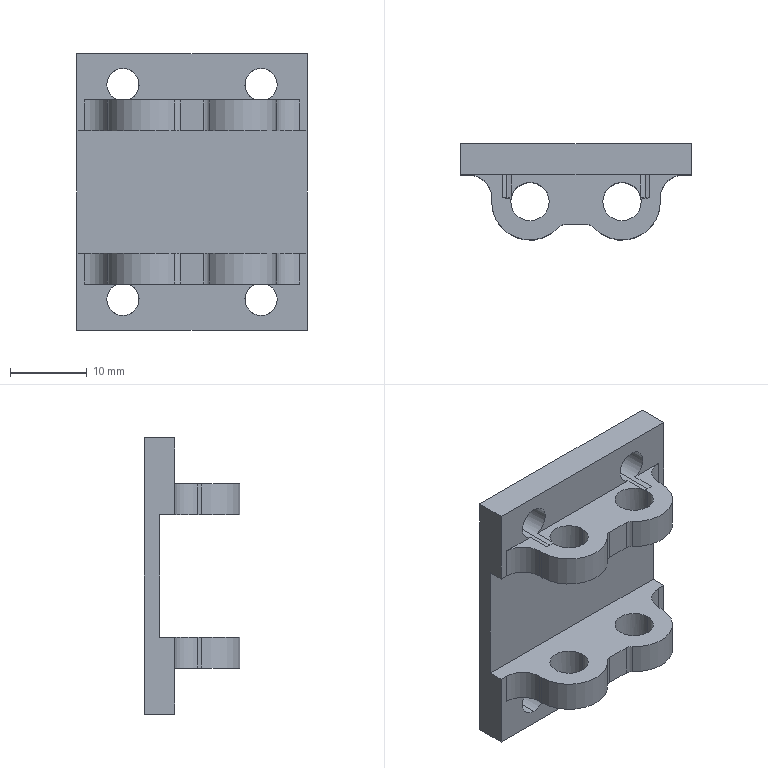Part | SolidWorks | features ICE 12, RevCut 4, Fillet 2, HoleWzd 2, BaseBody 1 | 1 solid | 52 faces | box 30 x 12.5 x 36 mm | volume 4162 mm3 | cylinder 28 | plane 18 | cone 6 | commonest cylinder face diameters 4.2 x8 5 x8 2 x4 6 x4 10 x4